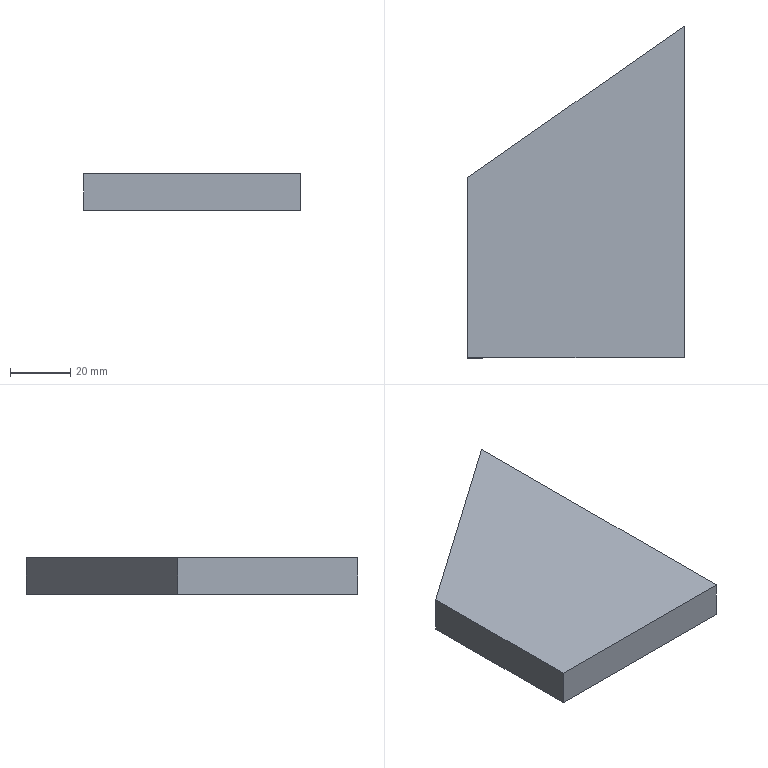Part | SolidWorks | features Extrusion 1 | 1 solid | 6 faces | box 72 x 110.415 x 12 mm | volume 73619 mm3 | plane 6
STEP:
#1=CARTESIAN_POINT('',(-30.,235.996,-260.));
#2=VERTEX_POINT('',#1);
#3=CARTESIAN_POINT('',(-102.,185.581,-260.));
#4=VERTEX_POINT('',#3);
#5=CARTESIAN_POINT('',(-102.,185.581,-260.));
#6=DIRECTION('',(-0.8192,-0.5736,0.));
#7=VECTOR('',#6,1000.);
#8=LINE('',#5,#7);
#9=EDGE_CURVE('',#2,#4,#8,.T.);
#10=ORIENTED_EDGE('',*,*,#9,.T.);
#11=CARTESIAN_POINT('',(-102.,185.581,-248.));
#12=VERTEX_POINT('',#11);
#13=CARTESIAN_POINT('',(-102.,185.581,-248.));
#14=DIRECTION('',(0.,0.,-1.));
#15=VECTOR('',#14,1000.);
#16=LINE('',#13,#15);
#17=EDGE_CURVE('',#12,#4,#16,.T.);
#18=ORIENTED_EDGE('',*,*,#17,.F.);
#19=CARTESIAN_POINT('',(-30.,235.996,-248.));
#20=VERTEX_POINT('',#19);
#21=CARTESIAN_POINT('',(-102.,185.581,-248.));
#22=DIRECTION('',(-0.8192,-0.5736,0.));
#23=VECTOR('',#22,1000.);
#24=LINE('',#21,#23);
#25=EDGE_CURVE('',#20,#12,#24,.T.);
#26=ORIENTED_EDGE('',*,*,#25,.F.);
#27=CARTESIAN_POINT('',(-30.,235.996,-248.));
#28=DIRECTION('',(0.,0.,-1.));
#29=VECTOR('',#28,1000.);
#30=LINE('',#27,#29);
#31=EDGE_CURVE('',#20,#2,#30,.T.);
#32=ORIENTED_EDGE('',*,*,#31,.T.);
#33=EDGE_LOOP('',(#10,#18,#26,#32));
#34=FACE_OUTER_BOUND('',#33,.T.);
#35=CARTESIAN_POINT('',(-102.,185.581,-248.));
#36=DIRECTION('',(0.5736,-0.8192,0.));
#37=DIRECTION('',(0.8192,0.5736,0.));
#38=AXIS2_PLACEMENT_3D('',#35,#36,#37);
#39=PLANE('',#38);
#40=ADVANCED_FACE('',(#34),#39,.F.);
#41=CARTESIAN_POINT('',(-102.,125.581,-260.));
#42=VERTEX_POINT('',#41);
#43=CARTESIAN_POINT('',(-102.,125.581,-260.));
#44=DIRECTION('',(0.,-1.,0.));
#45=VECTOR('',#44,1000.);
#46=LINE('',#43,#45);
#47=EDGE_CURVE('',#4,#42,#46,.T.);
#48=ORIENTED_EDGE('',*,*,#47,.T.);
#49=CARTESIAN_POINT('',(-102.,125.581,-248.));
#50=VERTEX_POINT('',#49);
#51=CARTESIAN_POINT('',(-102.,125.581,-248.));
#52=DIRECTION('',(0.,0.,-1.));
#53=VECTOR('',#52,1000.);
#54=LINE('',#51,#53);
#55=EDGE_CURVE('',#50,#42,#54,.T.);
#56=ORIENTED_EDGE('',*,*,#55,.F.);
#57=CARTESIAN_POINT('',(-102.,125.581,-248.));
#58=DIRECTION('',(0.,-1.,0.));
#59=VECTOR('',#58,1000.);
#60=LINE('',#57,#59);
#61=EDGE_CURVE('',#12,#50,#60,.T.);
#62=ORIENTED_EDGE('',*,*,#61,.F.);
#63=ORIENTED_EDGE('',*,*,#17,.T.);
#64=EDGE_LOOP('',(#48,#56,#62,#63));
#65=FACE_OUTER_BOUND('',#64,.T.);
#66=CARTESIAN_POINT('',(-102.,125.581,-248.));
#67=DIRECTION('',(1.,0.,0.));
#68=DIRECTION('',(0.,1.,0.));
#69=AXIS2_PLACEMENT_3D('',#66,#67,#68);
#70=PLANE('',#69);
#71=ADVANCED_FACE('',(#65),#70,.F.);
#72=CARTESIAN_POINT('',(-30.,125.581,-260.));
#73=VERTEX_POINT('',#72);
#74=CARTESIAN_POINT('',(-30.,125.581,-260.));
#75=DIRECTION('',(1.,0.,0.));
#76=VECTOR('',#75,1000.);
#77=LINE('',#74,#76);
#78=EDGE_CURVE('',#42,#73,#77,.T.);
#79=ORIENTED_EDGE('',*,*,#78,.T.);
#80=CARTESIAN_POINT('',(-30.,125.581,-248.));
#81=VERTEX_POINT('',#80);
#82=CARTESIAN_POINT('',(-30.,125.581,-248.));
#83=DIRECTION('',(0.,0.,-1.));
#84=VECTOR('',#83,1000.);
#85=LINE('',#82,#84);
#86=EDGE_CURVE('',#81,#73,#85,.T.);
#87=ORIENTED_EDGE('',*,*,#86,.F.);
#88=CARTESIAN_POINT('',(-30.,125.581,-248.));
#89=DIRECTION('',(1.,0.,0.));
#90=VECTOR('',#89,1000.);
#91=LINE('',#88,#90);
#92=EDGE_CURVE('',#50,#81,#91,.T.);
#93=ORIENTED_EDGE('',*,*,#92,.F.);
#94=ORIENTED_EDGE('',*,*,#55,.T.);
#95=EDGE_LOOP('',(#79,#87,#93,#94));
#96=FACE_OUTER_BOUND('',#95,.T.);
#97=CARTESIAN_POINT('',(-30.,125.581,-248.));
#98=DIRECTION('',(0.,1.,0.));
#99=DIRECTION('',(0.,0.,1.));
#100=AXIS2_PLACEMENT_3D('',#97,#98,#99);
#101=PLANE('',#100);
#102=ADVANCED_FACE('',(#96),#101,.F.);
#103=CARTESIAN_POINT('',(-30.,235.996,-260.));
#104=DIRECTION('',(0.,1.,0.));
#105=VECTOR('',#104,1000.);
#106=LINE('',#103,#105);
#107=EDGE_CURVE('',#73,#2,#106,.T.);
#108=ORIENTED_EDGE('',*,*,#107,.T.);
#109=ORIENTED_EDGE('',*,*,#31,.F.);
#110=CARTESIAN_POINT('',(-30.,235.996,-248.));
#111=DIRECTION('',(0.,1.,0.));
#112=VECTOR('',#111,1000.);
#113=LINE('',#110,#112);
#114=EDGE_CURVE('',#81,#20,#113,.T.);
#115=ORIENTED_EDGE('',*,*,#114,.F.);
#116=ORIENTED_EDGE('',*,*,#86,.T.);
#117=EDGE_LOOP('',(#108,#109,#115,#116));
#118=FACE_OUTER_BOUND('',#117,.T.);
#119=CARTESIAN_POINT('',(-30.,235.996,-248.));
#120=DIRECTION('',(-1.,0.,0.));
#121=DIRECTION('',(0.,-1.,0.));
#122=AXIS2_PLACEMENT_3D('',#119,#120,#121);
#123=PLANE('',#122);
#124=ADVANCED_FACE('',(#118),#123,.F.);
#125=ORIENTED_EDGE('',*,*,#25,.T.);
#126=ORIENTED_EDGE('',*,*,#61,.T.);
#127=ORIENTED_EDGE('',*,*,#92,.T.);
#128=ORIENTED_EDGE('',*,*,#114,.T.);
#129=EDGE_LOOP('',(#125,#126,#127,#128));
#130=FACE_OUTER_BOUND('',#129,.T.);
#131=CARTESIAN_POINT('',(0.,0.,-248.));
#132=DIRECTION('',(0.,0.,-1.));
#133=DIRECTION('',(-1.,0.,0.));
#134=AXIS2_PLACEMENT_3D('',#131,#132,#133);
#135=PLANE('',#134);
#136=ADVANCED_FACE('',(#130),#135,.F.);
#137=ORIENTED_EDGE('',*,*,#9,.F.);
#138=ORIENTED_EDGE('',*,*,#107,.F.);
#139=ORIENTED_EDGE('',*,*,#78,.F.);
#140=ORIENTED_EDGE('',*,*,#47,.F.);
#141=EDGE_LOOP('',(#137,#138,#139,#140));
#142=FACE_OUTER_BOUND('',#141,.T.);
#143=CARTESIAN_POINT('',(0.,0.,-260.));
#144=DIRECTION('',(0.,0.,-1.));
#145=DIRECTION('',(-1.,0.,0.));
#146=AXIS2_PLACEMENT_3D('',#143,#144,#145);
#147=PLANE('',#146);
#148=ADVANCED_FACE('',(#142),#147,.T.);
#149=CLOSED_SHELL('',(#40,#71,#102,#124,#136,#148));
#150=MANIFOLD_SOLID_BREP('',#149);
#151=CARTESIAN_POINT('',(0.,0.,0.));
#152=DIRECTION('',(0.,0.,1.));
#153=DIRECTION('',(1.,0.,0.));
#154=AXIS2_PLACEMENT_3D('',#151,#152,#153);
#155=(LENGTH_UNIT()NAMED_UNIT(*)SI_UNIT(.MILLI.,.METRE.));
#156=UNCERTAINTY_MEASURE_WITH_UNIT(LENGTH_MEASURE(0.00001),#155,'','');
#157=(NAMED_UNIT(*)PLANE_ANGLE_UNIT()SI_UNIT($,.RADIAN.));
#158=(NAMED_UNIT(*)SI_UNIT($,.STERADIAN.)SOLID_ANGLE_UNIT());
#159=(GEOMETRIC_REPRESENTATION_CONTEXT(3)GLOBAL_UNCERTAINTY_ASSIGNED_CONTEXT((#156))GLOBAL_UNIT_ASSIGNED_CONTEXT((#155,#157,#158))REPRESENTATION_CONTEXT('',''));
#160=ADVANCED_BREP_SHAPE_REPRESENTATION('',(#150,#154),#159);